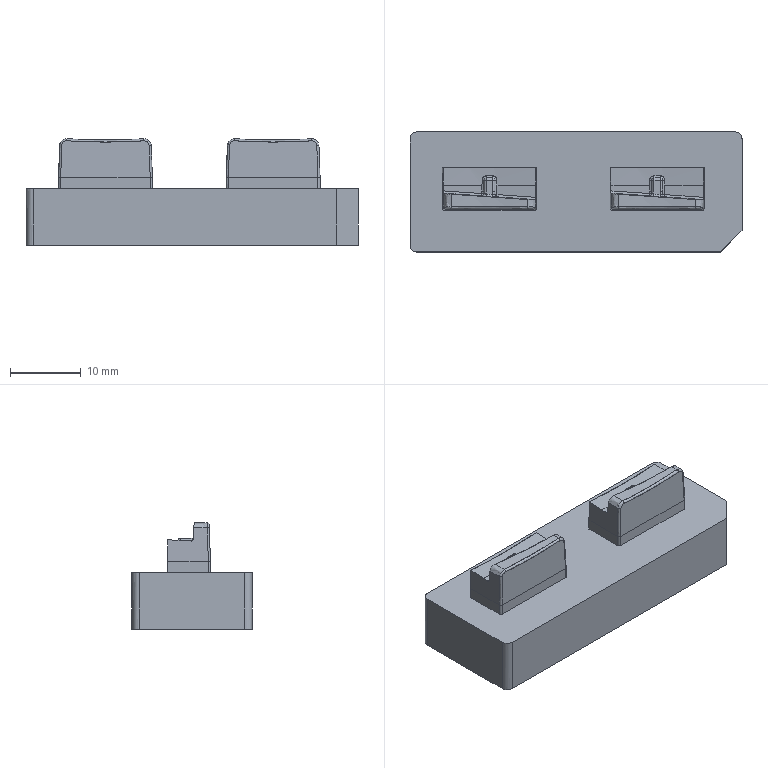NC program | PowerMill | posted with a generic post | part box 47 x 17 x 15.061 mm
Lines 8829 to 10132 of 128250:
N8926 M6
N8927 S22000 M03
N8928 G00 G90 X0.0 Y0.0
N8929 G43 Z9.8009 H27
N8930
N8931 G05 P10000 R4
N8932 X-5.329 Y-0.0692
N8933 Z-1.702
N8934 G01 Z-2.902 F1200.0
N8935 X-5.3385 Y-0.0592 F2000.0
N8936 G03 X-5.5134 Y-0.0542 I-0.09 J-0.085
N8937 G01 X-5.5486 Y-0.0875
N8938 X-5.7899 Y-0.1204
N8939 X-5.9806 Y0.0
N8940 X-6.4941 Y0.5508
N8941 X-7.7154 Y-0.397
N8942 X-7.7158 Y-0.4108
N8943 G03 X-7.5961 Y-0.5384 I0.1236 J-0.0039
N8944 G01 X-6.0311 Y-0.5877
N8945 X-5.7899 Y-0.5228
N8946 X-5.5486 Y-0.5595
N8947 X-5.3867 Y-0.7237
N8948 X-5.3776 Y-0.7813
N8949 G00 Z2.8222
N8950 G01 X-8.5986 Y-0.3083 F10000.0
N8951 G00 Z-1.7519
N8952 G01 Z-2.9519 F1200.0
N8953 X-8.5994 Y-0.322 F2000.0
N8954 G03 X-8.4824 Y-0.4522 I0.1236 J-0.0066
N8955 G01 X-8.2023 Y-0.4671
N8956 X-7.0249 Y-0.4811
N8957 X-7.0109 Y-0.4771
N8958 X-6.9985 Y-0.4715
N8959 X-6.9882 Y-0.4627
N8960 X-6.9878 Y-0.4622
N8961 X-6.9805 Y-0.4508
N8962 X-6.9768 Y-0.4377
N8963 X-6.9767 Y-0.4372
N8964 X-6.9769 Y-0.4236
N8965 X-6.981 Y-0.4106
N8966 X-6.9873 Y-0.3975
N8967 X-7.6515 Y0.334
N8968 G00 Z2.7323
N8969 G01 X-15.0794 Y0.0717 F10000.0
N8970 G00 Z-1.4527
N8971 G01 Z-2.6527 F1200.0
N8972 X-15.0804 Y0.058 F2000.0
N8973 G03 X-14.9657 Y-0.0742 I0.1234 J-0.0087
N8974 G01 X-13.5712 Y-0.1726
N8975 X-13.3667 Y-0.183
N8976 X-13.3554 Y-0.1822
N8977 X-13.3446 Y-0.1787
N8978 Y-0.1786
N8979 X-13.3355 Y-0.1731
N8980 X-13.3279 Y-0.1656
N8981 X-13.3273 Y-0.165
N8982 X-13.3216 Y-0.156
N8983 X-13.318 Y-0.146
N8984 X-13.3154 Y-0.1346
N8985 X-13.3145 Y1.301
N8986 G00 Z2.8637
N8987 G01 X-15.1224 Y0.0799 F10000.0
N8988 G00 Z-1.5026
N8989 G01 Z-2.7026 F1200.0
N8990 X-15.1233 Y0.0662 F2000.0
N8991 G03 X-15.0089 Y-0.0662 I0.1234 J-0.009
N8992 G01 X-13.4666 Y-0.178
N8993 X-13.4041 Y-0.1811
N8994 X-13.3933 Y-0.1804
N8995 X-13.3828 Y-0.1772
N8996 X-13.3822 Y-0.1769
N8997 X-13.3728 Y-0.1714
N8998 X-13.3649 Y-0.1639
N8999 X-13.3644 Y-0.1633
N9000 X-13.3585 Y-0.1542
N9001 X-13.3548 Y-0.144
N9002 X-13.3521 Y-0.1325
N9003 X-13.3534 Y1.4044
N9004 G00 Z2.8193
N9005 G01 X-15.1544 Y0.0864 F10000.0
N9006 G00 Z-1.5524
N9007 G01 Z-2.7524 F1200.0
N9008 X-15.1554 Y0.0727 F2000.0
N9009 G03 X-15.0411 Y-0.0599 I0.1234 J-0.0091
N9010 G01 X-13.4191 Y-0.1796
N9011 X-13.4055 Y-0.1769
N9012 X-13.3933 Y-0.1726
N9013 X-13.3828 Y-0.1652
N9014 X-13.3823 Y-0.1647
N9015 X-13.3742 Y-0.1547
N9016 X-13.3691 Y-0.1429
N9017 X-13.3654 Y-0.1295
N9018 X-13.3723 Y1.48
N9019 G00 Z2.7749
N9020 G01 X-15.1671 Y0.0913 F10000.0
N9021 G00 Z-1.6023
N9022 G01 Z-2.8023 F1200.0
N9023 X-15.1682 Y0.0775 F2000.0
N9024 G03 X-15.054 Y-0.0551 I0.1234 J-0.0092
N9025 G01 X-13.4328 Y-0.1769
N9026 X-13.4191 Y-0.1741
N9027 X-13.407 Y-0.1698
N9028 X-13.3964 Y-0.1624
N9029 X-13.396 Y-0.162
N9030 X-13.3878 Y-0.152
N9031 X-13.3827 Y-0.1402
N9032 X-13.379 Y-0.1268
N9033 X-13.3865 Y1.4978
N9034 G00 Z2.7305
N9035 G01 X-15.1843 Y0.0971 F10000.0
N9036 G00 Z-1.6522
N9037 G01 Z-2.8522 F1200.0
N9038 X-15.1853 Y0.0834 F2000.0
N9039 G03 X-15.0714 Y-0.0494 I0.1233 J-0.0094
N9040 G01 X-13.4426 Y-0.1743
N9041 X-13.4289 Y-0.1716
N9042 X-13.4167 Y-0.1673
N9043 X-13.4062 Y-0.1598
N9044 X-13.4057 Y-0.1594
N9045 X-13.3976 Y-0.1493
N9046 X-13.3925 Y-0.1375
N9047 X-13.3888 Y-0.124
N9048 X-13.4046 Y1.5001
N9049 G00 Z2.8658
N9050 G01 X-15.1952 Y0.1097 F10000.0
N9051 G00 Z-1.702
N9052 G01 Z-2.902 F1200.0
N9053 X-15.1962 Y0.096 F2000.0
N9054 G03 X-15.0825 Y-0.037 I0.1233 J-0.0096
N9055 G01 X-13.4566 Y-0.1641
N9056 X-13.4429 Y-0.1613
N9057 X-13.4307 Y-0.157
N9058 X-13.4201 Y-0.1495
N9059 X-13.4196 Y-0.1491
N9060 X-13.4115 Y-0.139
N9061 X-13.4064 Y-0.1271
N9062 X-13.4027 Y-0.1136
N9063 X-13.4233 Y1.5131
N9064 G00 Z2.8222
N9065 G01 X-15.1918 Y0.1586 F10000.0
N9066 G00 Z-1.7519
N9067 G01 Z-2.9519 F1200.0
N9068 X-15.1931 Y0.1449 F2000.0
N9069 G03 X-15.0816 Y0.01 I0.1232 J-0.0117
N9070 G01 X-13.4803 Y-0.1426
N9071 X-13.4663 Y-0.1399
N9072 X-13.4537 Y-0.1356
N9073 X-13.4428 Y-0.1279
N9074 X-13.4424 Y-0.1275
N9075 X-13.4341 Y-0.1171
N9076 X-13.4291 Y-0.1048
N9077 X-13.4256 Y-0.0909
N9078 X-13.4857 Y1.488
N9079 G00 Z1.4778
N9080 G01 X-18.05 Y1.1509 F10000.0
N9081 G00 Z-1.6522
N9082 G01 Z-2.8522 F1200.0
N9083 X-18.066 Y1.1649 F2000.0
N9084 G03 X-18.3358 Y1.147 I-0.1259 J-0.1439
N9085 G01 X-18.4952 Y0.965
N9086 X-18.5758 Y0.8921
N9087 X-18.8171 Y0.8208
N9088 X-18.9581 Y0.8847
N9089 X-19.3212 Y-0.0196
N9090 X-19.3088 Y-0.0254
N9091 G03 X-19.1442 Y0.0342 I0.0525 J0.1121
N9092 G01 X-19.0583 Y0.2176
N9093 X-18.8171 Y0.3276
N9094 X-17.4492 Y0.1591
N9095 X-17.2991 Y1.1369 Z-2.902
N9096 X-17.3093 Y1.1462
N9097 G03 X-17.4841 Y1.1378 I-0.0832 J-0.0916
N9098 G01 X-18.171 Y0.3819
N9099 X-18.1771 Y0.3699
N9100 X-18.1813 Y0.3582
N9101 X-18.1822 Y0.3457
N9102 X-18.1821 Y0.3451
N9103 X-18.1797 Y0.3328
N9104 X-18.1742 Y0.3217
N9105 X-18.1738 Y0.3211
N9106 X-18.1656 Y0.3118
N9107 X-18.1551 Y0.3049
N9108 X-18.143 Y0.2991
N9109 X-17.8263 Y0.2412
N9110 X-16.6497 Y0.1041
N9111 X-16.2218 Y0.7883 Z-2.9519
N9112 X-16.2348 Y0.8
N9113 G03 X-16.4572 Y0.7883 I-0.1054 J-0.117
N9114 G01 X-16.903 Y0.293
N9115 X-16.9091 Y0.2809
N9116 X-16.9132 Y0.269
N9117 X-16.9139 Y0.2564
N9118 Y0.2557
N9119 X-16.9113 Y0.2434
N9120 X-16.9056 Y0.2323
N9121 X-16.9052 Y0.2317
N9122 X-16.8967 Y0.2225
N9123 X-16.886 Y0.2158
N9124 X-16.8736 Y0.2102
N9125 X-16.4046 Y0.136
N9126 X-15.9214 Y0.09
N9127 G00 Z5.6544
N9128 G01 X-13.872 Y0.3522 F10000.0
N9129 G00 Z-2.8517
N9130 G01 X-13.9688 Y0.3875 Z-2.8535 F1200.0
N9131 X-14.2215 Y0.5995 Z-2.8593
N9132 X-14.3865 Y0.8853 Z-2.8651
N9133 X-14.4438 Y1.2102 Z-2.8708
N9134 X-14.3865 Y1.5351 Z-2.8766
N9135 X-14.2215 Y1.8208 Z-2.8823
N9136 X-13.9688 Y2.0329 Z-2.8881
N9137 X-13.6588 Y2.1458 Z-2.8939
N9138 X-13.4085 Z-2.8982
N9139 X-13.5086 Y1.9433 Z-2.9022
N9140 X-13.5114 Y1.9343 Z-2.9023
N9141 X-13.5463 Y1.693 Z-2.9066
N9142 X-13.5466 Y1.6873 Z-2.9067
N9143 X-13.5238 Y1.2088 Z-2.915
N9144 X-13.4792 Y0.2746 Z-2.9314
N9145 X-13.6588 Z-2.9345
N9146 X-13.9688 Y0.3875 Z-2.9403
N9147 X-14.2215 Y0.5995 Z-2.946
N9148 X-14.3865 Y0.8853 Z-2.9518
N9149 X-14.4438 Y1.2102 Z-2.9575
N9150 X-14.3865 Y1.5351 Z-2.9633
N9151 X-14.2215 Y1.8208 Z-2.969
N9152 X-13.9688 Y2.0329 Z-2.9748
N9153 X-13.6588 Y2.1458 Z-2.9806
N9154 X-13.4085 Z-2.9849
N9155 X-13.5086 Y1.9433 Z-2.9889
N9156 X-13.5114 Y1.9343 Z-2.989
N9157 X-13.5463 Y1.693 Z-2.9933
N9158 X-13.5466 Y1.6873 Z-2.9934
N9159 X-13.5238 Y1.2088 Z-3.0017
N9160 X-13.4938 Y1.2102
N9161 X-13.9569 Y1.1939 F2000.0
N9162 X-13.9637 Y1.3863
N9163 G03 X-14.2077 Y1.5166 I-0.1598 J-0.0056
N9164 G01 X-15.2055 Y0.8989
N9165 X-15.4556 Y0.7531
N9166 G03 X-15.4061 Y0.5285 I0.0608 J-0.1044
N9167 G01 X-14.1552 Y0.4104
N9168 G03 X-13.9366 Y0.6165 I0.0188 J0.1991
N9169 G01 X-13.9569 Y1.1939
N9170 X-13.4938 Y1.2102
N9171 X-13.5166 Y1.6887
N9172 X-13.4817 Y1.93
N9173 X-13.3624 Y2.1712
N9174 X-13.2632 Y2.2796
N9175 G03 X-13.3053 Y2.3631 I-0.0368 J0.0337
N9176 G01 X-13.5097 Y2.3415
N9177 X-13.9922 Y2.1925
N9178 X-15.4396 Y1.2952
N9179 X-15.6809 Y1.1632
N9180 X-15.9238 Y0.965
N9181 X-16.5561 Y0.2736
N9182 X-16.5665 Y0.2234
N9183 X-16.5272 Y0.1905
N9184 X-16.1634 Y0.1317
N9185 X-13.4871 Y-0.127
N9186 X-13.4478 Y-0.1134
N9187 X-13.4324 Y-0.0747
N9188 X-13.4361 Y0.0
N9189 X-13.4938 Y1.2102
N9190 X-13.7766 Y1.1581 Z-2.9016
N9191 X-13.629 Y1.2332 Z-2.9045 F1200.0
N9192 X-13.6001 Y1.2179 Z-2.9051
N9193 X-13.5679 Y0.9623 Z-2.9096
N9194 X-13.5416 Y0.479 Z-2.918
N9195 X-13.5154 Y-0.0016 Z-2.9264
N9196 Y-0.0017
N9197 X-13.5135 Y-0.0356 Z-2.927
N9198 X-13.5352 Y-0.0566 Z-2.9275
N9199 X-14.3226 Y0.0141 Z-2.9413
N9200 X-14.4043 Y0.1557 Z-2.9442
N9201 X-14.4616 Y0.4806 Z-2.9499
N9202 X-14.4043 Y0.8055 Z-2.9557
N9203 X-14.3773 Y0.8524 Z-2.9566
N9204 X-13.629 Y1.2332 Z-2.9713
N9205 X-13.6001 Y1.2179 Z-2.9719
N9206 X-13.5679 Y0.9623 Z-2.9764
N9207 X-13.5416 Y0.479 Z-2.9848
N9208 X-13.5154 Y-0.0016 Z-2.9932
N9209 Y-0.0017
N9210 X-13.5135 Y-0.0356 Z-2.9938
N9211 X-13.5352 Y-0.0566 Z-2.9943
N9212 X-14.3226 Y0.0141 Z-3.0081
N9213 X-14.4043 Y0.1557 Z-3.011
N9214 X-14.4616 Y0.4806 Z-3.0167
N9215 X-14.4043 Y0.8055 Z-3.0225
N9216 X-14.3773 Y0.8524 Z-3.0234
N9217 X-13.629 Y1.2332 Z-3.0381
N9218 X-13.6001 Y1.2179 Z-3.0387
N9219 X-13.5679 Y0.9623 Z-3.0432
N9220 X-13.5416 Y0.479 Z-3.0516
N9221 X-13.5116 Y0.4806
N9222 X-13.9997 F2000.0
N9223 X-14.0247 Y0.5056
N9224 X-14.0497 Y0.4806
N9225 X-14.0247 Y0.4556
N9226 X-13.9997 Y0.4806
N9227 X-13.5116
N9228 X-13.538 Y0.965
N9229 X-13.5703 Y1.2217
N9230 X-13.5965 Y1.2596
N9231 X-13.6426 Y1.26
N9232 X-15.6509 Y0.2378
N9233 X-15.6775 Y0.1848
N9234 X-15.6349 Y0.1437
N9235 X-14.7159 Y0.0193
N9236 X-13.5379 Y-0.0865
N9237 X-13.4987 Y-0.0727
N9238 X-13.4835 Y-0.0339
N9239 X-13.4854 Y0.0
N9240 X-13.5116 Y0.4806
N9241 X-13.5794 Y0.0818 Z-2.9515
N9242 X-13.6095 Y0.275 Z-2.9549 F1200.0
N9243 X-13.6194 Y0.2893 Z-2.9552
N9244 X-13.6384 Y0.2897 Z-2.9555
N9245 X-14.017 Y0.0936 Z-2.963
N9246 X-14.01 Y0.0559 Z-2.9636
N9247 X-13.5937 Y0.0093 Z-2.9709
N9248 X-13.5717 Y0.0322 Z-2.9715
N9249 X-13.6095 Y0.275 Z-2.9758
N9250 X-13.6194 Y0.2893 Z-2.9761
N9251 X-13.6384 Y0.2897 Z-2.9764
N9252 X-14.017 Y0.0936 Z-2.9839
N9253 X-14.01 Y0.0559 Z-2.9845
N9254 X-13.5937 Y0.0093 Z-2.9918
N9255 X-13.5717 Y0.0322 Z-2.9924
N9256 X-13.6095 Y0.275 Z-2.9967
N9257 X-13.6194 Y0.2893 Z-2.997
N9258 X-13.6384 Y0.2897 Z-2.9973
N9259 X-14.017 Y0.0936 Z-3.0048
N9260 X-14.01 Y0.0559 Z-3.0054
N9261 X-13.5937 Y0.0093 Z-3.0127
N9262 X-13.5717 Y0.0322 Z-3.0133
N9263 X-13.6095 Y0.275 Z-3.0176
N9264 X-13.6194 Y0.2893 Z-3.0179
N9265 X-13.6384 Y0.2897 Z-3.0182
N9266 X-14.017 Y0.0936 Z-3.0257
N9267 X-14.01 Y0.0559 Z-3.0263
N9268 X-13.5937 Y0.0093 Z-3.0336
N9269 X-13.5717 Y0.0322 Z-3.0342
N9270 X-13.6095 Y0.275 Z-3.0385
N9271 X-13.6194 Y0.2893 Z-3.0388
N9272 X-13.6384 Y0.2897 Z-3.0391
N9273 X-14.017 Y0.0936 Z-3.0465
N9274 X-14.01 Y0.0559 Z-3.0472
N9275 X-13.5937 Y0.0093 Z-3.0545
N9276 X-13.5717 Y0.0322 Z-3.0551
N9277 X-13.6095 Y0.275 Z-3.0594
N9278 X-13.6194 Y0.2893 Z-3.0597
N9279 X-13.6384 Y0.2897 Z-3.06
N9280 X-14.017 Y0.0936 Z-3.0674
N9281 X-14.01 Y0.0559 Z-3.0681
N9282 X-13.5937 Y0.0093 Z-3.0754
N9283 X-13.5717 Y0.0322 Z-3.076
N9284 X-13.6095 Y0.275 Z-3.0803
N9285 X-13.6194 Y0.2893 Z-3.0806
N9286 X-13.6384 Y0.2897 Z-3.0809
N9287 X-14.017 Y0.0936 Z-3.0883
N9288 X-14.01 Y0.0559 Z-3.089
N9289 X-13.5937 Y0.0093 Z-3.0963
N9290 X-13.5717 Y0.0322 Z-3.0969
N9291 X-13.6095 Y0.275 Z-3.1012
N9292 X-13.6194 Y0.2893 Z-3.1015
N9293 X-13.6047 Y0.3155
N9294 X-13.6284 Y0.3219 F2000.0
N9295 X-13.6522 Y0.3163
N9296 X-14.0308 Y0.1202
N9297 G03 X-14.0133 Y0.0261 I0.023 J-0.0444
N9298 G01 X-13.597 Y-0.0206
N9299 X-13.5554 Y-0.0055
N9300 X-13.5421 Y0.0368
N9301 X-13.5798 Y0.2796
N9302 X-13.5881 Y0.3004
N9303 X-13.6047 Y0.3155
N9304 G00 Z2.7323
N9305 G01 X-11.0505 Y1.0281 F10000.0
N9306 G00 Z-1.4527
N9307 G01 Z-2.6527 F1200.0
N9308 X-11.0642 Y1.0282 F2000.0
N9309 G03 X-11.1889 Y0.9053 I-0.0009 J-0.1238
N9310 G01 X-11.1973 Y-0.2891
N9311 X-11.1944 Y-0.3012
N9312 X-11.1904 Y-0.3119
N9313 X-11.1839 Y-0.3213
N9314 X-11.1834 Y-0.3218
N9315 X-11.1749 Y-0.3294
N9316 X-11.1647 Y-0.3347
N9317 X-11.1531 Y-0.3391
N9318 X-11.0972 Y-0.3456
N9319 X-9.7828 Y-0.4375
N9320 G00 Z2.6871
N9321 G01 X-11.0174 Y1.1457 F10000.0
N9322 G00 Z-1.5026
N9323 G01 Z-2.7026 F1200.0
N9324 X-11.0311 Y1.1458 F2000.0
N9325 G03 X-11.1553 Y1.0225 I-0.0005 J-0.1238
N9326 G01 X-11.1603 Y-0.2922
N9327 X-11.1572 Y-0.3046
N9328 X-11.1529 Y-0.3155
N9329 X-11.146 Y-0.3251
N9330 X-11.1455 Y-0.3256
N9331 X-11.1365 Y-0.3331
N9332 X-11.1259 Y-0.3382
N9333 X-11.1138 Y-0.3422
N9334 X-9.7356 Y-0.438
N9335 G00 Z2.8193
N9336 G01 X-11.0012 Y1.2192 F10000.0
N9337 G00 Z-1.5524
N9338 G01 Z-2.7524 F1200.0
N9339 X-11.015 Y1.2194 F2000.0
N9340 G03 X-11.1411 Y1.0981 I-0.0023 J-0.1237
N9341 G01 X-11.1481 Y0.3968
N9342 X-11.1428 Y-0.3044
N9343 X-11.1385 Y-0.3153
N9344 X-11.1316 Y-0.3248
N9345 X-11.1311 Y-0.3254
N9346 X-11.1221 Y-0.3329
N9347 X-11.1115 Y-0.3379
N9348 X-11.0994 Y-0.3419
N9349 X-9.7071 Y-0.4383
N9350 G00 Z2.7749
N9351 G01 X-10.9846 Y1.216 F10000.0
N9352 G00 Z-1.6023
N9353 G01 Z-2.8023 F1200.0
N9354 X-10.9984 Y1.2161 F2000.0
N9355 G03 X-11.123 Y1.0933 I-0.0009 J-0.1237
N9356 G01 X-11.1333 Y-0.2907
N9357 X-11.1302 Y-0.3031
N9358 X-11.1259 Y-0.3141
N9359 X-11.1191 Y-0.3237
N9360 X-11.1186 Y-0.3243
N9361 X-11.1095 Y-0.3318
N9362 X-11.0988 Y-0.3369
N9363 X-11.0867 Y-0.3409
N9364 X-9.6957 Y-0.4342
N9365 G00 Z2.7305
N9366 G01 X-10.9681 Y1.2209 F10000.0
N9367 G00 Z-1.6522
N9368 G01 Z-2.8522 F1200.0
N9369 X-10.9818 Y1.221 F2000.0
N9370 G03 X-11.107 Y1.0987 I-0.0015 J-0.1237
N9371 G01 X-11.1235 Y-0.2892
N9372 X-11.1204 Y-0.3017
N9373 X-11.1162 Y-0.3127
N9374 X-11.1093 Y-0.3224
N9375 X-11.1088 Y-0.3229
N9376 X-11.0997 Y-0.3305
N9377 X-11.089 Y-0.3356
N9378 X-11.0767 Y-0.3396
N9379 X-9.6813 Y-0.4288
N9380 G00 Z2.8658
N9381 G01 X-10.9511 Y1.23 F10000.0
N9382 G00 Z-1.702
N9383 G01 Z-2.902 F1200.0
N9384 X-10.9648 Y1.2302 F2000.0
N9385 G03 X-11.0905 Y1.1084 I-0.0019 J-0.1238
N9386 G01 X-11.1122 Y-0.2826
N9387 X-11.1092 Y-0.2951
N9388 X-11.1049 Y-0.3062
N9389 X-11.098 Y-0.3159
N9390 X-11.0975 Y-0.3164
N9391 X-11.0884 Y-0.3241
N9392 X-11.0777 Y-0.3292
N9393 X-11.0655 Y-0.3332
N9394 X-9.6697 Y-0.4239
N9395 G00 Z2.8222
N9396 G01 X-10.8943 Y1.2191 F10000.0
N9397 G00 Z-1.7519
N9398 G01 Z-2.9519 F1200.0
N9399 X-10.908 Y1.2196 F2000.0
N9400 G03 X-11.0365 Y1.1008 I-0.0049 J-0.1236
N9401 G01 X-11.0896 Y-0.2642
N9402 X-11.0867 Y-0.277
N9403 X-11.0825 Y-0.2884
N9404 X-11.0756 Y-0.2984
N9405 X-11.0751 Y-0.2989
N9406 X-11.0658 Y-0.3068
N9407 X-11.0548 Y-0.312
N9408 X-11.0423 Y-0.316
N9409 X-9.6419 Y-0.3905
N9410 G00 Z3.6763
N9411 G01 X-10.9655 Y1.5816 F10000.0
N9412 G00 Z-2.8517
N9413 G01 X-10.9651 Y1.5898 Z-2.8519 F1200.0
N9414 X-10.875 Z-2.8535
N9415 X-10.565 Y1.4769 Z-2.8592
N9416 X-10.3123 Y1.2648 Z-2.865
N9417 X-10.1473 Y0.9791 Z-2.8707
N9418 X-10.09 Y0.6542 Z-2.8765
N9419 X-10.1473 Y0.3293 Z-2.8823
N9420 X-10.3123 Y0.0435 Z-2.888
N9421 X-10.565 Y-0.1685 Z-2.8938
N9422 X-10.875 Y-0.2814 Z-2.8995
N9423 X-10.8922 Z-2.8998
N9424 X-11.0346 Y-0.2742 Z-2.9023
N9425 X-11.0535 Y-0.2532 Z-2.9028
N9426 X-11.01 Y0.6528 Z-2.9186
N9427 X-10.9651 Y1.5898 Z-2.935
N9428 X-10.875 Z-2.9366
N9429 X-10.565 Y1.4769 Z-2.9423
N9430 X-10.3123 Y1.2648 Z-2.9481
N9431 X-10.1473 Y0.9791 Z-2.9539
N9432 X-10.09 Y0.6542 Z-2.9596
N9433 X-10.1473 Y0.3293 Z-2.9654
N9434 X-10.3123 Y0.0435 Z-2.9711
N9435 X-10.565 Y-0.1685 Z-2.9769
N9436 X-10.875 Y-0.2814 Z-2.9826
N9437 X-10.8922 Z-2.9829
N9438 X-11.0346 Y-0.2742 Z-2.9854
N9439 X-11.0535 Y-0.2532 Z-2.9859
N9440 X-11.01 Y0.6528 Z-3.0017
N9441 X-11.04 Y0.6542
N9442 X-10.5648 F2000.0
N9443 X-10.0714
N9444 X-10.0489 Y0.6317
N9445 X-10.0264 Y0.6542
N9446 X-10.0489 Y0.6767
N9447 X-10.0714 Y0.6542
N9448 X-10.5648
N9449 X-10.5727 Y0.3496
N9450 G03 X-10.3853 Y0.1448 I0.1999 J-0.0052
N9451 G01 X-8.6627 Y0.037
N9452 G03 X-8.5722 Y0.2617 I0.008 J0.1274
N9453 G01 X-9.0294 Y0.6485
N9454 X-10.2807 Y1.4184
N9455 G03 X-10.5487 Y1.2731 I-0.0922 J-0.1499
N9456 G01 X-10.5648 Y0.6542
N9457 X-11.04
N9458 X-11.0835 Y-0.2518
N9459 X-11.0706 Y-0.2877
N9460 X-11.0361 Y-0.3041
N9461 X-7.9611 Y-0.4602
N9462 X-7.4101 Y-0.4564
N9463 X-7.3646 Y-0.4265
N9464 X-7.3734 Y-0.3729
N9465 X-7.4927 Y-0.2412
N9466 X-8.6848 Y1.074
N9467 X-9.3711 Y1.4475
N9468 X-9.3736 Y1.4816
N9469 X-9.3975 Y1.5061
N9470 X-10.3735 Y1.9757
N9471 X-11.0636 Y2.2169
N9472 X-11.0874 Y2.2192
N9473 X-11.1095 Y2.2102
N9474 X-11.133 Y2.1813
N9475 X-11.13 Y2.1442
N9476 X-11.0234 Y1.93
N9477 X-10.9904 Y1.6887
N9478 X-11.04 Y0.6542
N9479 X-9.0823 Y0.2614 Z-2.9016
N9480 X-9.1537 Y0.1377 Z-2.9041 F1200.0
N9481 X-9.4065 Y-0.0743 Z-2.9099
N9482 X-9.7165 Y-0.1872 Z-2.9156
N9483 X-10.0464 Z-2.9214
N9484 X-10.3565 Y-0.0743 Z-2.9271
N9485 X-10.6092 Y0.1377 Z-2.9329
N9486 X-10.7742 Y0.4235 Z-2.9386
N9487 X-10.8315 Y0.7484 Z-2.9444
N9488 X-10.7742 Y1.0733 Z-2.9502
N9489 X-10.7279 Y1.1535 Z-2.9518
N9490 X-9.8953 Y0.7218 Z-2.9681
N9491 X-9.0651 Y0.2913 Z-2.9845
N9492 X-9.1537 Y0.1377 Z-2.9876
N9493 X-9.4065 Y-0.0743 Z-2.9933
N9494 X-9.7165 Y-0.1872 Z-2.9991
N9495 X-10.0464 Z-3.0048
N9496 X-10.3565 Y-0.0743 Z-3.0106
N9497 X-10.6092 Y0.1377 Z-3.0164
N9498 X-10.7742 Y0.4235 Z-3.0221
N9499 X-10.8315 Y0.7484 Z-3.0279
N9500 X-10.7742 Y1.0733 Z-3.0336
N9501 X-10.7279 Y1.1535 Z-3.0352
N9502 X-9.8953 Y0.7218 Z-3.0516
N9503 X-9.8815 Y0.7484
N9504 X-10.0775 Y0.3308 F2000.0
N9505 X-10.3253 Y0.4471
N9506 G03 X-10.5324 Y0.3509 I-0.0633 J-0.1347
N9507 G03 X-10.4012 Y0.164 I0.1438 J-0.0385
N9508 G01 X-10.1284 Y0.1408
N9509 G03 X-10.0775 Y0.3308 I0.0084 J0.0996
N9510 G01 X-9.8815 Y0.7484
N9511 X-10.8638 Y1.2578
N9512 X-10.9095 Y1.2579
N9513 X-10.9363 Y1.2208
N9514 X-10.9748 Y0.965
N9515 X-11.0387 Y-0.2185
N9516 X-11.026 Y-0.2545
N9517 X-10.9916 Y-0.2711
N9518 X-9.6498 Y-0.3484
N9519 X-8.3418 Y-0.376
N9520 X-8.2953 Y-0.3468
N9521 X-8.3036 Y-0.2926
N9522 X-8.3499 Y-0.2412
N9523 X-8.6848 Y0.1279
N9524 X-9.8815 Y0.7484
N9525 X-10.388 Y-0.2163 Z-2.9515
N9526 X-9.9517 Y-0.2355 Z-2.9591 F1200.0
N9527 X-9.9416 Y-0.1978 Z-2.9598
N9528 X-10.283 Y-0.0191 Z-2.9665
N9529 X-10.8704 Y0.2882 Z-2.9781
N9530 X-10.8996 Y0.2728 Z-2.9786
N9531 X-10.9523 Y-0.1699 Z-2.9864
N9532 X-10.9333 Y-0.1922 Z-2.9869
N9533 X-9.9517 Y-0.2355 Z-3.0041
N9534 X-9.9416 Y-0.1978 Z-3.0048
N9535 X-10.283 Y-0.0191 Z-3.0115
N9536 X-10.8704 Y0.2882 Z-3.0231
N9537 X-10.8996 Y0.2728 Z-3.0236
N9538 X-10.9523 Y-0.1699 Z-3.0314
N9539 X-10.9333 Y-0.1922 Z-3.0319
N9540 X-9.9517 Y-0.2355 Z-3.0491
N9541 X-9.9416 Y-0.1978 Z-3.0498
N9542 X-10.283 Y-0.0191 Z-3.0565
N9543 X-10.8704 Y0.2882 Z-3.068
N9544 X-10.8996 Y0.2728 Z-3.0686
N9545 X-10.9523 Y-0.1699 Z-3.0764
N9546 X-10.9333 Y-0.1922 Z-3.0769
N9547 X-9.9517 Y-0.2355 Z-3.0941
N9548 X-9.9416 Y-0.1978 Z-3.0947
N9549 X-10.283 Y-0.0191 Z-3.1015
N9550 X-10.2691 Y0.0074
N9551 X-10.8565 Y0.3148 F2000.0
N9552 X-10.903 Y0.3147
N9553 X-10.9293 Y0.2764
N9554 X-10.9821 Y-0.1663
N9555 X-10.9705 Y-0.2046
N9556 X-10.9346 Y-0.2222
N9557 X-9.953 Y-0.2655
N9558 G03 X-9.9276 Y-0.1712 I0.0022 J0.05
N9559 G01 X-10.2691 Y0.0074
N9560 G00 Z2.9095
N9561 G01 X5.6983 Y1.153 F10000.0
N9562 G00 Z-1.6522
N9563 G01 Z-2.8522 F1200.0
N9564 X5.6826 Y1.1673 F2000.0
N9565 G03 X5.4124 Y1.1538 I-0.1283 J-0.1418
N9566 G01 X5.2416 Y0.965
N9567 X5.0661 Y0.8393
N9568 X4.8249 Y0.8414
N9569 X4.784 Y0.8806
N9570 X4.4128 Y-0.0109
N9571 X4.4248 Y-0.0176
N9572 G03 X4.5933 Y0.0296 I0.0606 J0.1079
N9573 G01 X4.7123 Y0.2412
N9574 X4.8249 Y0.3065
N9575 X5.0661 Y0.3124
N9576 X6.3084 Y0.1523
N9577 X6.4574 Y1.1558 Z-2.902
N9578 X6.4472 Y1.165
N9579 G03 X6.2724 Y1.1562 I-0.083 J-0.0918
N9580 G01 X5.5725 Y0.3818
N9581 X5.5664 Y0.3698
N9582 X5.5623 Y0.358
N9583 X5.5614 Y0.3456
N9584 Y0.345
N9585 X5.5638 Y0.3327
N9586 X5.5693 Y0.3216
N9587 X5.5697 Y0.321
N9588 X5.578 Y0.3117
N9589 X5.5884 Y0.3049
N9590 X5.6005 Y0.2991
N9591 X6.0311 Y0.2199
N9592 X7.1331 Y0.0985
N9593 X7.4984 Y0.8097 Z-2.9519
N9594 X7.4882 Y0.819
N9595 G03 X7.3134 Y0.8108 I-0.0833 J-0.0915
N9596 G01 X6.8423 Y0.2936
N9597 X6.8361 Y0.2815
N9598 X6.8319 Y0.2695
N9599 X6.8311 Y0.2569
N9600 X6.8312 Y0.2562
N9601 X6.8337 Y0.2439
N9602 X6.8395 Y0.2326
N9603 X6.8399 Y0.2321
N9604 X6.8485 Y0.2228
N9605 X6.8592 Y0.2161
N9606 X6.8717 Y0.2105
N9607 X7.4786 Y0.1179
N9608 X7.8776 Y0.0806
N9609 G00 Z2.9081
N9610 G01 X8.6556 Y0.0712 F10000.0
N9611 G00 Z-1.4527
N9612 G01 Z-2.6527 F1200.0
N9613 X8.6547 Y0.0575 F2000.0
N9614 G03 X8.7695 Y-0.0746 I0.1234 J-0.0086
N9615 G01 X10.2455 Y-0.1778
N9616 X10.3779 Y-0.1847
N9617 X10.3998 Y-0.1805
N9618 X10.4174 Y-0.1666
N9619 X10.4175 Y-0.1665
N9620 X10.423 Y-0.1576
N9621 X10.4263 Y-0.1477
N9622 X10.4288 Y-0.1366
N9623 X10.423 Y1.2922
N9624 G00 Z2.8637
N9625 G01 X8.6176 Y0.0812 F10000.0
N9626 G00 Z-1.5026
N9627 G01 Z-2.7026 F1200.0
N9628 X8.6166 Y0.0675 F2000.0
N9629 G03 X8.731 Y-0.0649 I0.1234 J-0.009
N9630 G01 X10.3383 Y-0.1824
N9631 X10.3519 Y-0.1796
N9632 X10.364 Y-0.1753
N9633 X10.3745 Y-0.1679
N9634 X10.375 Y-0.1675
N9635 X10.3831 Y-0.1576
N9636 X10.3882 Y-0.1458
N9637 X10.3919 Y-0.1324
N9638 X10.3906 Y1.4199
N9639 G00 Z2.8193
N9640 G01 X8.5932 Y0.0865 F10000.0
N9641 G00 Z-1.5524
N9642 G01 Z-2.7524 F1200.0
N9643 X8.5921 Y0.0728 F2000.0
N9644 G03 X8.7064 Y-0.0598 I0.1235 J-0.0092
N9645 G01 X10.3249 Y-0.1796
N9646 X10.3385 Y-0.1769
N9647 X10.3506 Y-0.1726
N9648 X10.3611 Y-0.1652
N9649 X10.3616 Y-0.1648
N9650 X10.3697 Y-0.1548
N9651 X10.3749 Y-0.143
N9652 X10.3786 Y-0.1297
N9653 X10.377 Y1.2062
N9654 X10.3732 Y1.4886
N9655 G00 Z2.7749
N9656 G01 X8.5708 Y0.0889 F10000.0
N9657 G00 Z-1.6023
N9658 G01 Z-2.8023 F1200.0
N9659 X8.5697 Y0.0752 F2000.0
N9660 G03 X8.6831 Y-0.0581 I0.1234 J-0.0099
N9661 G01 X9.5036 Y-0.1202
N9662 X10.3246 Y-0.1743
N9663 X10.3368 Y-0.17
N9664 X10.3473 Y-0.1626
N9665 X10.3477 Y-0.1621
N9666 X10.3558 Y-0.1522
N9667 X10.3609 Y-0.1403
N9668 X10.3646 Y-0.127
N9669 X10.3574 Y1.497
N9670 G00 Z2.7305
N9671 G01 X8.5684 Y0.101 F10000.0
N9672 G00 Z-1.6522
N9673 G01 Z-2.8522 F1200.0
N9674 X8.5674 Y0.0873 F2000.0
N9675 G03 X8.681 Y-0.0459 I0.1233 J-0.0098
N9676 G01 X10.3005 Y-0.1741
N9677 X10.3142 Y-0.1714
N9678 X10.3265 Y-0.1671
N9679 X10.3371 Y-0.1597
N9680 X10.3375 Y-0.1593
N9681 X10.3457 Y-0.1492
N9682 X10.3508 Y-0.1373
N9683 X10.3545 Y-0.1238
N9684 X10.3394 Y1.4984
N9685 G00 Z2.8658
N9686 G01 X8.5464 Y0.108 F10000.0
N9687 G00 Z-1.702
N9688 G01 Z-2.902 F1200.0
N9689 X8.5454 Y0.0943 F2000.0
N9690 G03 X8.6592 Y-0.0386 I0.1233 J-0.0095
N9691 G01 X10.2875 Y-0.1641
N9692 X10.3012 Y-0.1614
N9693 X10.3134 Y-0.1571
N9694 X10.324 Y-0.1496
N9695 X10.3245 Y-0.1492
N9696 X10.3326 Y-0.1391
N9697 X10.3377 Y-0.1271
N9698 X10.3413 Y-0.1136
N9699 X10.3203 Y1.5107
N9700 G00 Z2.8222
N9701 G01 X8.5479 Y0.1559 F10000.0
N9702 G00 Z-1.7519
N9703 G01 Z-2.9519 F1200.0
N9704 X8.5466 Y0.1423 F2000.0
N9705 G03 X8.6583 Y0.0075 I0.1232 J-0.0116
N9706 G01 X10.2639 Y-0.1427
N9707 X10.2779 Y-0.14
N9708 X10.2905 Y-0.1356
N9709 X10.3013 Y-0.128
N9710 X10.3017 Y-0.1276
N9711 X10.31 Y-0.1172
N9712 X10.315 Y-0.1049
N9713 X10.3185 Y-0.091
N9714 X10.2583 Y1.4865
N9715 G00 Z3.2655
N9716 G01 X8.6975 Y1.4432 F10000.0
N9717 G00 Z-2.8517
N9718 G01 X8.9395 Y1.5913 Z-2.8567 F1200.0
N9719 X9.0152 Y1.6215 Z-2.8581
N9720 X9.0702 Y1.5263 Z-2.86
N9721 X9.1275 Y1.2014 Z-2.8658
N9722 X9.0702 Y0.8764 Z-2.8716
N9723 X8.9052 Y0.5907 Z-2.8773
N9724 X8.6525 Y0.3786 Z-2.8831
N9725 X8.3424 Y0.2658 Z-2.8888
N9726 X8.0125 Z-2.8946
N9727 X7.7025 Y0.3786 Z-2.9003
N9728 X7.4906 Y0.5564 Z-2.9052
N9729 X7.9758 Y1.0817 Z-2.9177
N9730 X7.9827 Y1.0865 Z-2.9178
N9731 X8.1891 Y1.1737 Z-2.9217
N9732 X8.2007 Y1.1786 Z-2.9219
N9733 X8.2048 Y1.1807 Z-2.922
N9734 X8.4572 Y1.3371 Z-2.9272
N9735 X8.6584 Y1.4197 Z-2.931
N9736 X8.6626 Y1.4219 Z-2.9311
N9737 X8.9395 Y1.5913 Z-2.9367
N9738 X9.0152 Y1.6215 Z-2.9382
N9739 X9.0702 Y1.5263 Z-2.9401
N9740 X9.1275 Y1.2014 Z-2.9458
N9741 X9.0702 Y0.8764 Z-2.9516
N9742 X8.9052 Y0.5907 Z-2.9574
N9743 X8.6525 Y0.3786 Z-2.9631
N9744 X8.3424 Y0.2658 Z-2.9689
N9745 X8.0125 Z-2.9746
N9746 X7.7025 Y0.3786 Z-2.9804
N9747 X7.4906 Y0.5564 Z-2.9852
N9748 X7.9758 Y1.0817 Z-2.9977
N9749 X7.9827 Y1.0865 Z-2.9978
N9750 X8.1891 Y1.1737 Z-3.0017
N9751 X8.1775 Y1.2014
N9752 X8.3424 Y0.773 F2000.0
N9753 X8.2825 Y0.7499
N9754 G03 X8.3117 Y0.5341 I0.0402 J-0.1044
N9755 G01 X9.5878 Y0.408
N9756 G03 X9.8074 Y0.6136 I0.0197 J0.1991
N9757 G01 X9.7861 Y1.2634
N9758 G03 X9.523 Y1.4054 I-0.1729 J-0.0057
N9759 G01 X9.2788 Y1.2562
N9760 X9.0772 Y1.1391
N9761 X8.8705 Y1.0311
N9762 X8.3624 Y0.7806
N9763 X8.3424 Y0.773
N9764 X8.1775 Y1.2014
N9765 X7.971 Y1.1142
N9766 X7.9617 Y1.109
N9767 X7.9537 Y1.102
N9768 X7.1887 Y0.2739
N9769 X7.1782 Y0.2237
N9770 X7.2174 Y0.1906
N9771 X7.7198 Y0.1092
N9772 X10.2572 Y-0.1273
N9773 X10.2962 Y-0.1138
N9774 X10.3118 Y-0.0757
N9775 X10.3091 Y0.0
N9776 X10.2273 Y1.6887
N9777 X10.2622 Y1.93
N9778 X10.3735 Y2.1606
N9779 X10.5889 Y2.3564
N9780 G03 X10.543 Y2.4419 I-0.0337 J0.037
N9781 G01 X10.426 Y2.4124
N9782 X9.9786 Y2.1712
N9783 X9.6498 Y2.0087
N9784 X9.5392 Y1.93
N9785 X9.1673 Y1.7485
N9786 X9.1025 Y1.6887
N9787 X8.926 Y1.6182
N9788 X8.647 Y1.4475
N9789 X8.4436 Y1.3639
N9790 X8.189 Y1.2062
N9791 X8.1775 Y1.2014
N9792 G00 Z3.5925
N9793 G01 X9.993 Y1.1785 F10000.0
N9794 G00 Z-2.9016
N9795 G01 X10.1145 Y1.238 Z-2.904 F1200.0
N9796 X10.1431 Y1.2226 Z-2.9045
N9797 X10.176 Y0.9623 Z-2.9091
N9798 X10.2026 Y0.4772 Z-2.9176
N9799 X10.2289 Y-0.0015 Z-2.926
N9800 X10.2305 Y-0.0359 Z-2.9266
N9801 X10.2087 Y-0.0567 Z-2.9271
N9802 X9.4211 Y0.0131 Z-2.9409
N9803 X9.3399 Y0.1539 Z-2.9437
N9804 X9.2826 Y0.4788 Z-2.9495
N9805 X9.3399 Y0.8038 Z-2.9552
N9806 X9.3764 Y0.8671 Z-2.9565
N9807 X9.4213 Y0.8938 Z-2.9574
N9808 X9.545 Y0.9366 Z-2.9597
N9809 X9.5522 Y0.9402 Z-2.9599
N9810 X9.6649 Y1.0176 Z-2.9622
N9811 X10.1145 Y1.238 Z-2.971
N9812 X10.1431 Y1.2226 Z-2.9715
N9813 X10.176 Y0.9623 Z-2.9761
N9814 X10.2026 Y0.4772 Z-2.9846
N9815 X10.2289 Y-0.0015 Z-2.993
N9816 X10.2305 Y-0.0359 Z-2.9936
N9817 X10.2087 Y-0.0567 Z-2.9941
N9818 X9.4211 Y0.0131 Z-3.0079
N9819 X9.3399 Y0.1539 Z-3.0107
N9820 X9.2826 Y0.4788 Z-3.0165
N9821 X9.3399 Y0.8038 Z-3.0222
N9822 X9.3764 Y0.8671 Z-3.0235
N9823 X9.4213 Y0.8938 Z-3.0244
N9824 X9.545 Y0.9366 Z-3.0267
N9825 X9.5522 Y0.9402 Z-3.0269
N9826 X9.6649 Y1.0176 Z-3.0292
N9827 X10.1145 Y1.238 Z-3.038
N9828 X10.1431 Y1.2226 Z-3.0386
N9829 X10.176 Y0.9623 Z-3.0431
N9830 X10.2026 Y0.4772 Z-3.0516
N9831 X10.2326 Y0.4788
N9832 X9.7447 F2000.0
N9833 X9.7179 Y0.5056
N9834 X9.6912 Y0.4788
N9835 X9.7179 Y0.4521
N9836 X9.7447 Y0.4788
N9837 X10.2326
N9838 X10.2059 Y0.965
N9839 X10.1729 Y1.2264
N9840 X10.147 Y1.2641
N9841 X10.1013 Y1.265
N9842 X9.6498 Y1.0436
N9843 X9.5352 Y0.965
N9844 X9.4085 Y0.9212
N9845 X9.0775 Y0.7237
N9846 X8.926 Y0.6668
N9847 X8.1241 Y0.2412
N9848 X8.0791 Y0.1922
N9849 X8.1226 Y0.1419
N9850 X9.1673 Y0.0055
N9851 X10.2061 Y-0.0866
N9852 X10.2451 Y-0.0729
N9853 X10.2605 Y-0.0344
N9854 X10.2588 Y0.0
N9855 X10.2326 Y0.4788
N9856 X10.1637 Y0.0911 Z-2.9515
N9857 X10.1346 Y0.2751 Z-2.9547 F1200.0
N9858 X10.1248 Y0.2893 Z-2.955
N9859 X10.1057 Y0.2897 Z-2.9554
N9860 X9.7269 Y0.0935 Z-2.9628
N9861 X9.7339 Y0.0559 Z-2.9635
N9862 X10.1511 Y0.0092 Z-2.9708
N9863 X10.1731 Y0.0322 Z-2.9713
N9864 X10.1346 Y0.2751 Z-2.9756
N9865 X10.1248 Y0.2893 Z-2.9759
N9866 X10.1057 Y0.2897 Z-2.9763
N9867 X9.7269 Y0.0935 Z-2.9837
N9868 X9.7339 Y0.0559 Z-2.9844
N9869 X10.1511 Y0.0092 Z-2.9917
N9870 X10.1731 Y0.0322 Z-2.9923
N9871 X10.1346 Y0.2751 Z-2.9966
N9872 X10.1248 Y0.2893 Z-2.9969
N9873 X10.1057 Y0.2897 Z-2.9972
N9874 X9.7269 Y0.0935 Z-3.0046
N9875 X9.7339 Y0.0559 Z-3.0053
N9876 X10.1511 Y0.0092 Z-3.0126
N9877 X10.1731 Y0.0322 Z-3.0132
N9878 X10.1346 Y0.2751 Z-3.0175
N9879 X10.1248 Y0.2893 Z-3.0178
N9880 X10.1057 Y0.2897 Z-3.0181
N9881 X9.7269 Y0.0935 Z-3.0256
N9882 X9.7339 Y0.0559 Z-3.0262
N9883 X10.1511 Y0.0092 Z-3.0336
N9884 X10.1731 Y0.0322 Z-3.0341
N9885 X10.1346 Y0.2751 Z-3.0384
N9886 X10.1248 Y0.2893 Z-3.0387
N9887 X10.1057 Y0.2897 Z-3.039
N9888 X9.7269 Y0.0935 Z-3.0465
N9889 X9.7339 Y0.0559 Z-3.0472
N9890 X10.1511 Y0.0092 Z-3.0545
N9891 X10.1731 Y0.0322 Z-3.055
N9892 X10.1346 Y0.2751 Z-3.0593
N9893 X10.1248 Y0.2893 Z-3.0596
N9894 X10.1057 Y0.2897 Z-3.06
N9895 X9.7269 Y0.0935 Z-3.0674
N9896 X9.7339 Y0.0559 Z-3.0681
N9897 X10.1511 Y0.0092 Z-3.0754
N9898 X10.1731 Y0.0322 Z-3.076
N9899 X10.1346 Y0.2751 Z-3.0802
N9900 X10.1248 Y0.2893 Z-3.0805
N9901 X10.1057 Y0.2897 Z-3.0809
N9902 X9.7269 Y0.0935 Z-3.0883
N9903 X9.7339 Y0.0559 Z-3.089
N9904 X10.1511 Y0.0092 Z-3.0963
N9905 X10.1731 Y0.0322 Z-3.0969
N9906 X10.1346 Y0.2751 Z-3.1012
N9907 X10.1248 Y0.2893 Z-3.1015
N9908 X10.1396 Y0.3154
N9909 X10.1159 Y0.3219 F2000.0
N9910 X10.0919 Y0.3163
N9911 X9.7131 Y0.1202
N9912 G03 X9.7306 Y0.0261 I0.023 J-0.0444
N9913 G01 X10.1478 Y-0.0207
N9914 X10.1895 Y-0.0055
N9915 X10.2027 Y0.0368
N9916 X10.1643 Y0.2798
N9917 X10.156 Y0.3004
N9918 X10.1396 Y0.3154
N9919 G00 Z2.7323
N9920 G01 X12.69 Y1.0318 F10000.0
N9921 G00 Z-1.4527
N9922 G01 Z-2.6527 F1200.0
N9923 X12.6762 F2000.0
N9924 G03 X12.5519 Y0.9087 I-0.0005 J-0.1237
N9925 G01 X12.5464 Y-0.29
N9926 X12.5492 Y-0.3019
N9927 X12.553 Y-0.3123
N9928 X12.5592 Y-0.3216
N9929 X12.5597 Y-0.3222
N9930 X12.568 Y-0.3297
N9931 X12.5777 Y-0.3351
N9932 X12.589 Y-0.3397
N9933 X12.6133 Y-0.3434
N9934 X13.9611 Y-0.438
N9935 G00 Z2.6871
N9936 G01 X12.7272 Y1.145 F10000.0
N9937 G00 Z-1.5026
N9938 G01 Z-2.7026 F1200.0
N9939 X12.7134 Y1.1451 F2000.0
N9940 G03 X12.5892 Y1.0218 I-0.0005 J-0.1238
N9941 G01 X12.5836 Y-0.2918
N9942 X12.5868 Y-0.3042
N9943 X12.591 Y-0.3152
N9944 X12.5979 Y-0.3248
N9945 X12.5984 Y-0.3253
N9946 X12.6074 Y-0.3328
N9947 X12.6181 Y-0.3379
N9948 X12.6302 Y-0.3419
N9949 X14.007 Y-0.4365
N9950 G00 Z2.8193
N9951 G01 X12.7452 Y1.2028 F10000.0
N9952 G00 Z-1.5524
N9953 G01 Z-2.7524 F1200.0
N9954 X12.7315 Y1.2029 F2000.0
N9955 G03 X12.607 Y1.0799 I-0.0008 J-0.1238
N9956 G01 X12.5983 Y-0.2915
N9957 X12.6014 Y-0.3039
N9958 X12.6057 Y-0.3149
N9959 X12.6126 Y-0.3245
N9960 X12.6131 Y-0.325
N9961 X12.6221 Y-0.3326
N9962 X12.6328 Y-0.3377
N9963 X12.645 Y-0.3417
N9964 X14.0293 Y-0.4334
N9965 G00 Z2.7749
N9966 G01 X12.7582 Y1.2148 F10000.0
N9967 G00 Z-1.6023
N9968 G01 Z-2.8023 F1200.0
N9969 X12.7445 Y1.2149 F2000.0
N9970 G03 X12.6199 Y1.092 I-0.0009 J-0.1237
N9971 G01 X12.6106 Y-0.2906
N9972 X12.6137 Y-0.303
N9973 X12.618 Y-0.314
N9974 X12.6249 Y-0.3236
N9975 X12.6254 Y-0.3241
N9976 X12.6344 Y-0.3317
N9977 X12.6451 Y-0.3368
N9978 X12.6573 Y-0.3408
N9979 X14.0467 Y-0.4323
N9980 G00 Z2.7305
N9981 G01 X12.7753 Y1.2212 F10000.0
N9982 G00 Z-1.6522
N9983 G01 Z-2.8522 F1200.0
N9984 X12.7615 Y1.2214 F2000.0
N9985 G03 X12.6363 Y1.099 I-0.0014 J-0.1238
N9986 G01 X12.6204 Y-0.2894
N9987 X12.6235 Y-0.3019
N9988 X12.6277 Y-0.313
N9989 X12.6346 Y-0.3226
N9990 X12.6351 Y-0.3232
N9991 X12.6442 Y-0.3308
N9992 X12.6549 Y-0.3359
N9993 X12.6671 Y-0.3399
N9994 X14.0666 Y-0.4306
N9995 G00 Z2.8658
N9996 G01 X12.7928 Y1.2307 F10000.0
N9997 G00 Z-1.702
N9998 G01 Z-2.902 F1200.0
N9999 X12.7791 Y1.2309 F2000.0
N10000 G03 X12.6534 Y1.1091 I-0.002 J-0.1238
N10001 G01 X12.6317 Y-0.2821
N10002 X12.6348 Y-0.2947
N10003 X12.639 Y-0.3058
N10004 X12.6459 Y-0.3155
N10005 X12.6464 Y-0.316
N10006 X12.6555 Y-0.3237
N10007 X12.6662 Y-0.3288
N10008 X12.6785 Y-0.3328
N10009 X14.0753 Y-0.424
N10010 G00 Z2.8222
N10011 G01 X12.8504 Y1.2185 F10000.0
N10012 G00 Z-1.7519
N10013 G01 Z-2.9519 F1200.0
N10014 X12.8367 Y1.2191 F2000.0
N10015 G03 X12.7081 Y1.1003 I-0.0049 J-0.1237
N10016 G01 X12.6544 Y-0.2638
N10017 X12.6573 Y-0.2767
N10018 X12.6615 Y-0.2881
N10019 X12.6684 Y-0.2981
N10020 X12.6689 Y-0.2986
N10021 X12.6782 Y-0.3065
N10022 X12.6893 Y-0.3117
N10023 X12.7018 Y-0.3157
N10024 X14.0958 Y-0.3853
N10025 G00 Z2.8658
N10026 G01 X16.0189 Y-0.3957 F10000.0
N10027 G00 Z-1.702
N10028 G01 Z-2.902 F1200.0
N10029 X16.0184 Y-0.4095 F2000.0
N10030 G03 X16.1377 Y-0.5375 I0.1237 J-0.0043
N10031 G01 X17.6108 Y-0.5891
N10032 X18.0933 Y-0.5237
N10033 X18.3346 Y-0.6845
N10034 X18.3631 Y-0.8181
N10035 X18.4002 Y-0.0943
N10036 X18.3929 Y-0.0827
N10037 G03 X18.2223 Y-0.0435 I-0.1049 J-0.0657
N10038 G01 X18.0933 Y-0.1243
N10039 X17.8521 Y-0.0835
N10040 X17.6108 Y0.1517
N10041 X17.5546 Y0.2412
N10042 X17.3696 Y0.4178
N10043 X17.3349 Y0.4825
N10044 X17.2594 Y0.5627
N10045 G00 Z2.8222
N10046 G01 X15.1566 Y-0.3006 F10000.0
N10047 G00 Z-1.7519
N10048 G01 Z-2.9519 F1200.0
N10049 X15.1559 Y-0.3143 F2000.0
N10050 G03 X15.2733 Y-0.4441 I0.1236 J-0.0062
N10051 G01 X16.1634 Y-0.4885
N10052 X16.7225 Y-0.4835
N10053 X16.7363 Y-0.4793
N10054 X16.7485 Y-0.4735
N10055 X16.7585 Y-0.4646
N10056 X16.7589 Y-0.4642
N10057 X16.766 Y-0.4527
N10058 X16.7696 Y-0.4398
N10059 X16.7697 Y-0.4392
N10060 X16.7694 Y-0.4258
N10061 X16.7654 Y-0.4129
N10062 X16.7591 Y-0.3999
N10063 X16.0974 Y0.3298
N10064 G00 Z3.6757
N10065 G01 X12.7782 Y1.5653 F10000.0
N10066 G00 Z-2.8517
N10067 G01 X12.7791 Y1.585 Z-2.8521 F1200.0
N10068 X12.8689 Z-2.8537
N10069 X13.1789 Y1.4722 Z-2.8594
N10070 X13.4317 Y1.2601 Z-2.8652
N10071 X13.5966 Y0.9743 Z-2.8709
N10072 X13.6539 Y0.6494 Z-2.8767
N10073 X13.5966 Y0.3245 Z-2.8825
N10074 X13.4317 Y0.0388 Z-2.8882
N10075 X13.1789 Y-0.1733 Z-2.894
N10076 X12.8795 Y-0.2823 Z-2.8995
N10077 X12.7094 Y-0.274 Z-2.9025
N10078 X12.6904 Y-0.2531 Z-2.903
N10079 X12.7339 Y0.648 Z-2.9187
N10080 X12.7791 Y1.585 Z-2.9351
N10081 X12.8689 Z-2.9367
N10082 X13.1789 Y1.4722 Z-2.9424
N10083 X13.4317 Y1.2601 Z-2.9482
N10084 X13.5966 Y0.9743 Z-2.9539
N10085 X13.6539 Y0.6494 Z-2.9597
N10086 X13.5966 Y0.3245 Z-2.9655
N10087 X13.4317 Y0.0388 Z-2.9712
N10088 X13.1789 Y-0.1733 Z-2.977
N10089 X12.8795 Y-0.2823 Z-2.9825
N10090 X12.7094 Y-0.274 Z-2.9855
N10091 X12.6904 Y-0.2531 Z-2.986
N10092 X12.7339 Y0.648 Z-3.0017
N10093 X12.7039 Y0.6494
N10094 X13.1791 F2000.0
N10095 X13.6658
N10096 X13.701 Y0.6142
N10097 X13.7362 Y0.6494
N10098 X13.701 Y0.6847
N10099 X13.6658 Y0.6494
N10100 X13.1791
N10101 X13.1713 Y0.351
N10102 G03 X13.3592 Y0.1462 I0.1999 J-0.0052
N10103 G01 X15.077 Y0.0428
N10104 G03 X15.1667 Y0.2682 I0.0077 J0.1275
N10105 G01 X14.7205 Y0.6409
N10106 X13.4669 Y1.4041
N10107 G03 X13.1948 Y1.2557 I-0.0931 J-0.1531
N10108 G01 X13.1791 Y0.6494
N10109 X12.7039
N10110 X12.6605 Y-0.2516
N10111 X12.6734 Y-0.2877
N10112 X12.708 Y-0.304
N10113 X15.9221 Y-0.4596
N10114 X16.3375 Y-0.4565
N10115 X16.3827 Y-0.4271
N10116 X16.3748 Y-0.3737
N10117 X16.2597 Y-0.2412
N10118 X15.0695 Y1.0621
N10119 X14.3828 Y1.4475
N10120 X14.2334 Y1.5614
N10121 X13.0272 Y2.1139
N10122 X12.6744 Y2.2102
N10123 X12.6225 Y2.1935
N10124 X12.6167 Y2.1393
N10125 X12.723 Y1.93
N10126 X12.7541 Y1.6887
N10127 X12.7039 Y0.6494
N10128 X14.6457 Y0.2636 Z-2.9016
N10129 X14.5754 Y0.1418 Z-2.9041 F1200.0
N10130 X14.3227 Y-0.0703 Z-2.9098
N10131 X14.0126 Y-0.1831 Z-2.9156
N10132 X13.6827 Z-2.9213
N10133 X13.3727 Y-0.0703 Z-2.9271
N10134 X13.1199 Y0.1418 Z-2.9329
N10135 X12.955 Y0.4275 Z-2.9386
N10136 X12.8977 Y0.7524 Z-2.9444
N10137 X12.955 Y1.0773 Z-2.9501
N10138 X13.0026 Y1.1598 Z-2.9518
N10139 X13.8338 Y0.7258 Z-2.9682
N10140 X14.6628 Y0.2931 Z-2.9845
N10141 X14.5754 Y0.1418 Z-2.9875
N10142 X14.3227 Y-0.0703 Z-2.9933
N10143 X14.0126 Y-0.1831 Z-2.999
N10144 X13.6827 Z-3.0048
N10145 X13.3727 Y-0.0703 Z-3.0106
N10146 X13.1199 Y0.1418 Z-3.0163
N10147 X12.955 Y0.4275 Z-3.0221
N10148 X12.8977 Y0.7524 Z-3.0278
N10149 X12.955 Y1.0773 Z-3.0336
N10150 X13.0026 Y1.1598 Z-3.0352
N10151 X13.8338 Y0.7258 Z-3.0516
N10152 X13.8477 Y0.7524
N10153 X13.6554 Y0.3328 F2000.0
N10154 X13.4162 Y0.4424
N10155 G03 X13.2181 Y0.3497 I-0.0597 J-0.1305
N10156 G03 X13.3417 Y0.1693 I0.1384 J-0.0378
N10157 G01 X13.6033 Y0.1422
N10158 G03 X13.6554 Y0.3328 I0.0104 J0.0996
N10159 G01 X13.8477 Y0.7524
N10160 X12.8781 Y1.2586
N10161 X12.8329 Y1.2592
N10162 X12.8057 Y1.2232
N10163 X12.786 Y1.1138
N10164 X12.7056 Y-0.2182
N10165 X12.7181 Y-0.2544
N10166 X12.7526 Y-0.2711
N10167 X14.2334 Y-0.3554
N10168 X15.4061 Y-0.3764
N10169 X15.4524 Y-0.3474
N10170 X15.4445 Y-0.2934
N10171 X15.3986 Y-0.2412
N10172 X15.0818 Y0.1082
N10173 X13.8477 Y0.7524
N10174 X13.3486 Y-0.215 Z-2.9515
N10175 X13.7854 Y-0.2335 Z-2.9591 F1200.0
N10176 X13.7955 Y-0.1958 Z-2.9598
N10177 X13.4462 Y-0.0125 Z-2.9667
N10178 X12.8689 Y0.2905 Z-2.978
N10179 X12.84 Y0.2769 Z-2.9786
N10180 X12.8157 Y0.1612 Z-2.9807
N10181 X12.7895 Y-0.1705 Z-2.9865
N10182 X12.8086 Y-0.192 Z-2.987
N10183 X13.7854 Y-0.2335 Z-3.004
N10184 X13.7955 Y-0.1958 Z-3.0047
N10185 X13.4462 Y-0.0125 Z-3.0116
N10186 X12.8689 Y0.2905 Z-3.023
N10187 X12.84 Y0.2769 Z-3.0235
N10188 X12.8157 Y0.1612 Z-3.0256
N10189 X12.7895 Y-0.1705 Z-3.0314
N10190 X12.8086 Y-0.192 Z-3.0319
N10191 X13.7854 Y-0.2335 Z-3.049
N10192 X13.7955 Y-0.1958 Z-3.0497
N10193 X13.4462 Y-0.0125 Z-3.0565
N10194 X12.8689 Y0.2905 Z-3.0679
N10195 X12.84 Y0.2769 Z-3.0685
N10196 X12.8157 Y0.1612 Z-3.0705
N10197 X12.7895 Y-0.1705 Z-3.0763
N10198 X12.8086 Y-0.192 Z-3.0768
N10199 X13.7854 Y-0.2335 Z-3.0939
N10200 X13.7955 Y-0.1958 Z-3.0946
N10201 X13.4462 Y-0.0125 Z-3.1015
N10202 X13.4602 Y0.0141
N10203 X12.8829 Y0.317 F2000.0
N10204 X12.8383 Y0.318
N10205 X12.8107 Y0.2831
N10206 X12.786 Y0.1655
N10207 X12.7596 Y-0.1681
N10208 X12.772 Y-0.2052
N10209 X12.8073 Y-0.222
N10210 X13.7841 Y-0.2635
N10211 X13.8345 Y-0.2265
N10212 X13.8095 Y-0.1693
N10213 X13.4602 Y0.0141
N10214 G00 Z9.8009
N10215 G05 P0
N10216 (---------------)
N10217 ( END TOOLPATH : 粗公再粗03-外形偏置-D1C )
N10218 (---------------)
N10219
N10220 M05
N10221 G53 Z0.0
N10222 (---------------)
N10223 ( START TOOLPATH : 粗公基准台01-基准面偏置-D10 )
N10224 (---------------)
N10225 ( TOOL NO.    :3 )
N10226 ( TOOL TYPE   : ENDMILL)
N10227 ( TOOL ID     : D10_1_1)
N10228 ( TOOL DIA    : 10.0 LENGTH 70.24)
N10229 T3